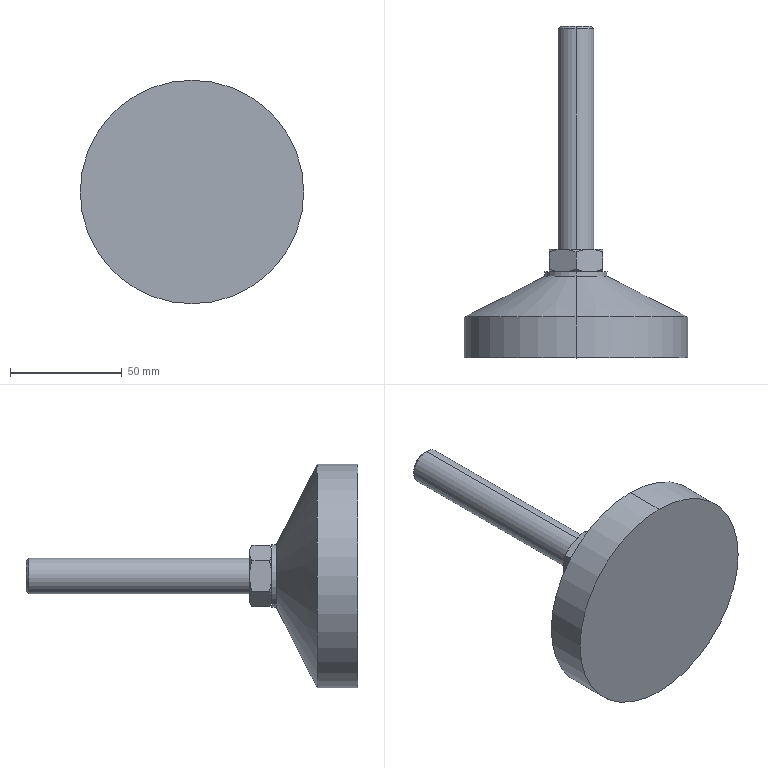Part | STEP file | 1 solid | 34 faces | box 100 x 148.5 x 100 mm | volume 234497 mm3 | cone 18 | plane 10 | cylinder 6 | commonest cylinder face diameters 16 x2 28 x2 100 x2